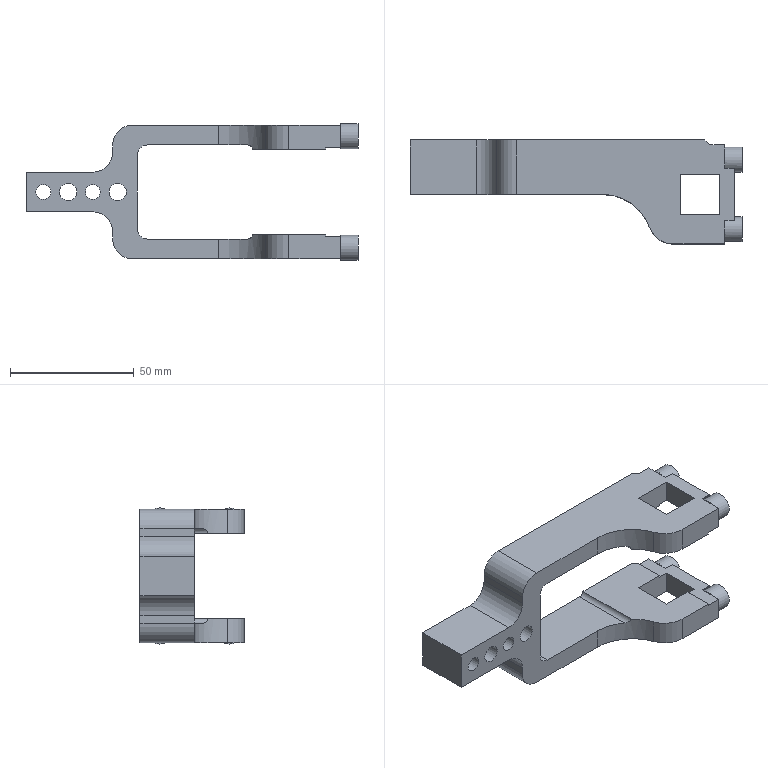Part | NX | features BREP 1 | 1 solid | 88 faces | box 134 x 42 x 55 mm | volume 63712 mm3 | plane 64 | cylinder 24 | commonest cylinder face diameters 10 x8 16 x4 4 x2 6 x2 7 x2 8 x2